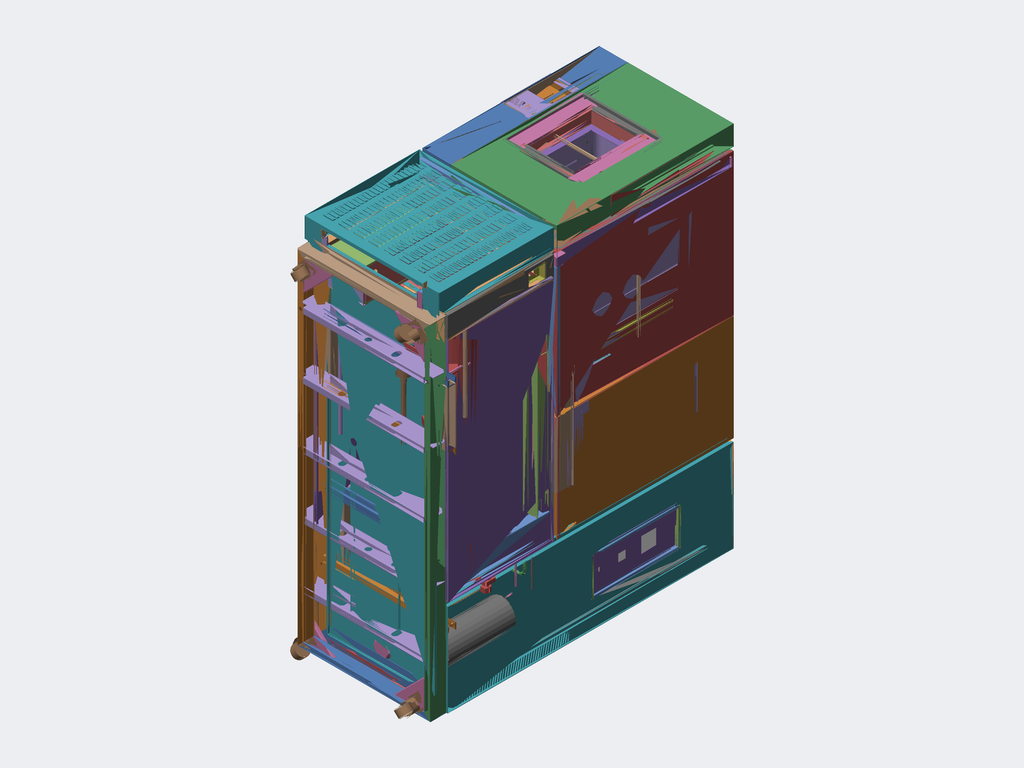Assembly | STEP file | 165 different items | 941 placed
Parts list (item | name | quantity | parent item | size | volume):
1 | HESS-408-70-15W-W-1-outer case side panel 1 | x1 | in HESS-408-70-15W-outer case assembly | 798.5 x 1049 x 630 mm | 1988997 mm3
2 | HESS-408-70-15W-W-2-outer case side panel 2 | x1 | in HESS-408-70-15W-outer case assembly | 798.5 x 1049 x 630 mm | 1938320 mm3
3 | HESS-408-70-15W-W-3-outer case side panel 3 | x1 | in HESS-408-70-15W-outer case assembly | 798.5 x 1049 x 850 mm | 2623190 mm3
4 | HESS-408-70-15W-W-4-outer case side panel 4 | x1 | in HESS-408-70-15W-outer case assembly | 798.5 x 1049 x 850 mm | 2624739 mm3
5 | HESS-408-70-15W-W-5-outer case reinforcing rib 1 | x1 | in HESS-408-70-15W-outer case assembly | 1043 x 80 x 20 mm | 296450 mm3
6 | HESS-408-70-15W-W-6-outer case reinforcing rib 2 | x1 | in HESS-408-70-15W-outer case assembly | 20 x 1043 x 80 mm | 295868 mm3
7 | HESS-408-70-15W-W-7-outer case reinforcing rib 3 | x2 | in HESS-408-70-15W-outer case assembly | 790 x 58.5 x 64 mm | 256348 mm3
8 | HESS-408-70-15W-W-8-outer case reinforcing rib 4 | x2 | in HESS-408-70-15W-outer case assembly | 45 x 930 x 20 mm | 171064 mm3
9 | HESS-408-70-15W-W-9-outer case triangular plate | x4 | in HESS-408-70-15W-outer case assembly | 60 x 60 x 4 mm | 2733 mm3
10 | HESS-408-70-15W-W-10-outer case rear closing plate | x1 | in HESS-408-70-15W-outer case assembly | 697 x 947 x 15 mm | 1092654 mm3
11 | HESS-408-70-15W-W-38-motor fixing bracket | x1 | in HESS-408-70-15W-outer case assembly | 795 x 36 x 250 mm | 812268 mm3
12 | HESS-408-70-15W-W-46-outer case reinforcing rib 5 | x2 | in HESS-408-70-15W-outer case assembly | 755 x 18.5 x 60 mm | 169016 mm3
13 | HESS-408-70-15W-W-47-outer case reinforcing rib 6 | x1 | in HESS-408-70-15W-outer case assembly | 670 x 18.5 x 34 mm | 97679 mm3
14 | HESS-408-70-15W-W-48-outer case reinforcing rib 7 | x2 | in HESS-408-70-15W-outer case assembly | 620 x 18 x 60 mm | 138005 mm3
15 | HESS-408-70-15W-N-1-inner liner upper cover | x1 | in HESS-408-70-15W-inner liner assembly | 650 x 790 x 1338 mm | 2883753 mm3
16 | HESS-408-70-15W-N-2-inner liner lower cover | x1 | in HESS-408-70-15W-inner liner assembly | 650 x 110 x 1338 mm | 1081692 mm3
17 | HESS-408-70-15W-N-3-inner liner rear panel | x1 | in HESS-408-70-15W-inner liner assembly | 600 x 864.78 x 10 mm | 539176 mm3
18 | HESS-408-70-15W-N-6-inner liner turbine outlet baffle | x1 | in HESS-408-70-15W-inner liner assembly | 600 x 69 x 169 mm | 141384 mm3
19 | HESS-408-70-15W-N-7-inner liner turbine panel | x1 | in HESS-408-70-15W-inner liner assembly | 492.743 x 461.634 x 1 mm | 101400 mm3
20 | HESS-408-70-15W-N-8-inner liner turbine enclosure plate | x1 | in HESS-408-70-15W-inner liner assembly | 512.743 x 461.634 x 144 mm | 193062 mm3
21 | HESS-408-70-15W-N-9-inner liner rounded corner | x4 | in HESS-408-70-15W-inner liner assembly | 55 x 55 x 1 mm | 2125 mm3
22 | HESS-408-70-15W-N-12-inner liner closing plate bracket Z | x1 | in HESS-408-70-15W-inner liner assembly | 30 x 657 x 20 mm | 34871 mm3
23 | HESS-408-70-15W-N-11-inner liner closing plate bracket Y | x1 | in HESS-408-70-15W-inner liner assembly | 30 x 657 x 20 mm | 34871 mm3
24 | HESS-408-70-15W-N-13-inner liner outer closing plate | x1 | in HESS-408-70-15W-inner liner assembly | 792 x 1042 x 2.5 mm | 754601 mm3
25 | HESS-408-70-15W-N-14-inner liner partition bracket | x4 | in HESS-408-70-15W-inner liner assembly | 12 x 600 x 42 mm | 43540 mm3
26 | HESS-408-70-15W-N-15-inner liner closing plate | x1 | in HESS-408-70-15W-inner liner assembly | 568 x 685 x 18 mm | 406764 mm3
27 | HESS-408-70-15W-N-16-inner liner louver left side panel | x1 | in HESS-408-70-15W-inner liner louver assembly | 40 x 194 x 15 mm | 10672 mm3
28 | HESS-408-70-15W-N-17-inner liner louver right side panel | x1 | in HESS-408-70-15W-inner liner louver assembly | 40 x 194 x 15 mm | 9821 mm3
29 | HESS-408-70-15W-N-18-inner liner louver blade | x8 | in HESS-408-70-15W-inner liner louver assembly | 516 x 19.734 x 14.16 mm | 12923 mm3
30 | HESS-408-70-15W-N-19-inner liner louver upper baffle | x1 | in HESS-408-70-15W-inner liner louver assembly | 519 x 20 x 2.1 mm | 18114 mm3
31 | HESS-408-70-15W-N-20-inner liner louver lower baffle | x1 | in HESS-408-70-15W-inner liner louver assembly | 519 x 20 x 25 mm | 26517 mm3
32 | HESS-408-70-15W-N-21-inner liner partition plate | x2 | in HESS-408-70-15W-inner liner partition plate assembly | - | 280081 mm3
33 | HESS-408-70-15W-N-22-inner liner partition plate reinforcing rib | x2 | in HESS-408-70-15W-inner liner partition plate assembly | 560 x 13 x 43 mm | 36943 mm3
34 | HESS-408-70-15W-N-23-inner liner bottom plate reinforcing plate 1 | x3 | in HESS-408-70-15W-inner liner assembly | 50 x 540 x 16.5 mm | 59626 mm3
35 | HESS-408-70-15W-D-6-electrical mounting plate bracket | x1 | in HESS-408-70-15W-electrical box assembly | 13 x 43 x 470 mm | 31006 mm3
36 | HESS-408-70-15W-D-4-electrical box bottom plate | x1 | in HESS-408-70-15W-electrical box assembly | 640 x 113.5 x 30 mm | 146678 mm3
37 | HESS-408-70-15W-D-11-frame panel | x1 | in HESS-408-70-15W-electrical box assembly | 1.5 x 520 x 220 mm | 155544 mm3
38 | HESS-408-70-15W-D-2-electrical box right side panel | x1 | in HESS-408-70-15W-electrical box assembly | 93.5 x 1699 x 568.5 mm | 1802522 mm3
39 | HESS-408-70-15W-D-7-electrical box door panel reinforcing rib | x1 | in HESS-408-70-15W-electrical box assembly | 77 x 1495 x 12.5 mm | 218735 mm3
40 | HESS-408-70-15W-D-5-electrical box door panel | x1 | in HESS-408-70-15W-electrical box assembly | 636 x 1516 x 14 mm | 1489085 mm3
41 | HESS-408-70-15W-D-12-electrical mounting plate | x1 | in HESS-408-70-15W-electrical box assembly | 520 x 1630 x 10 mm | 1311169 mm3
42 | HESS-408-70-15W-D-1-electrical box left side panel | x1 | in HESS-408-70-15W-electrical box assembly | 93.5 x 1699 x 568.5 mm | 1630922 mm3
43 | HESS-408-70-15W-D-3-electrical box top plate | x1 | in HESS-408-70-15W-electrical box assembly | 797 x 93.5 x 568.5 mm | 793198 mm3
44 | HESS-408-70-15W-D-10-edge strip 2 | x2 | in HESS-408-70-15W-electrical box frame assembly | 500 x 20 x 15 mm | 30917 mm3
45 | HESS-408-70-15W-D-9-edge strip 1 | x2 | in HESS-408-70-15W-electrical box frame assembly | 230 x 20 x 15 mm | 13161 mm3
46 | HESS-408-70-15W-D-8-electrical box lower closing plate | x1 | in HESS-408-70-15W-electrical box assembly | 200 x 95 x 3 mm | 41690 mm3
47 | HESS-408-70-15W-W-15-bottom frame 5 | x5 | in HESS-408-70-15W-base assembly | 785 x 100 x 50 mm | 395842 mm3
48 | HESS-408-70-15W-W-11-bottom frame 1 | x1 | in HESS-408-70-15W-base assembly | 790 x 100 x 100 mm | 538062 mm3
49 | HESS-408-70-15W-W-12-bottom frame 2 | x1 | in HESS-408-70-15W-base assembly | 790 x 100 x 100 mm | 531868 mm3
50 | HESS-408-70-15W-W-13-bottom frame 3 | x1 | in HESS-408-70-15W-base assembly | 100 x 100 x 2039 mm | 1445665 mm3
51 | HESS-408-70-15W-W-14-bottom frame 4 | x1 | in HESS-408-70-15W-base assembly | 100 x 100 x 2039 mm | 1445666 mm3
52 | HESS-408-70-15W-W-29-outer case lower support 4 | x1 | in HESS-408-70-15W-base assembly | 85 x 100 x 1180 mm | 851335 mm3
53 | HESS-408-70-15W-W-19-side door panel | x2 | in HESS-408-70-15W-base assembly | 18 x 629 x 1358 mm | 1424005 mm3
54 | HESS-408-70-15W-W-20-cabinet lower left outer plate | x1 | in HESS-408-70-15W-base assembly | 21.5 x 631 x 120 mm | 150313 mm3
55 | HESS-408-70-15W-W-18-bottom frame triangular plate | x4 | in HESS-408-70-15W-base assembly | 175 x 18 x 175 mm | 57661 mm3
56 | HESS-408-70-15W-W-21-cabinet lower right outer plate | x1 | in HESS-408-70-15W-base assembly | 21.5 x 631 x 120 mm | 138943 mm3
57 | HESS-408-70-15W-W-30-emergency stop switch box | x1 | in HESS-408-70-15W-base assembly | 35 x 114 x 94 mm | 21062 mm3
58 | HESS-408-70-15W-W-16-bottom frame drip tray 1 | x1 | in HESS-408-70-15W-base assembly | 2000 x 15 x 640 mm | 2094402 mm3
59 | HESS-408-70-15W-W-17-outer case lower support 1 | x1 | in HESS-408-70-15W-base assembly | 763 x 650 x 150 mm | 1372071 mm3
60 | HESS-408-70-15W-W-27-outer case lower support 2 | x1 | in HESS-408-70-15W-base assembly | 763 x 650 x 150 mm | 1289227 mm3
61 | HESS-408-70-15W-W-28-outer case lower support 3 | x1 | in HESS-408-70-15W-base assembly | 85 x 100 x 1180 mm | 851335 mm3
62 | door stop B | x2 | in HESS-408-70-15W-base assembly | 10 x 36.6 x 13.8 mm | 1298 mm3
63 | front lower door bracket-Z (SPCC-3.0) | x1 | in HESS-408-70-15W-base assembly | 30 x 40 x 87 mm | 14354 mm3
64 | copper tube 1_default_machined_ | x1 | in 408 quick-temperature-change freezer tray assembly | 388 x 422 x 519.8 mm | 116086 mm3
65 | VIB-C1-3-8-vibration damping pipe 35_default_machined_ | x2 | in 408 quick-temperature-change freezer tray assembly | 380 x 45 x 45 mm | 185668 mm3
66 | 4NES-14Y-40P | x1 | in 408 quick-temperature-change freezer tray assembly | - | -
67 | copper tube 3_default_machined_ | x1 | in 408 quick-temperature-change freezer tray assembly | 235 x 205.85 x 207.5 mm | 114578 mm3
68 | copper tube 5_default_machined_ | x1 | in 408 quick-temperature-change freezer tray assembly | 35 x 22 x 22 mm | 3381 mm3
69 | SGN22S-sight glass | x1 | in 408 quick-temperature-change freezer tray assembly | 173 x 36.5 x 29 mm | 27166 mm3
70 | three-quarters elbow_default_machined_ | x2 | in 408 quick-temperature-change freezer tray assembly | 35 x 19 x 35 mm | 3675 mm3
71 | copper tube 4_default_machined_ | x1 | in 408 quick-temperature-change freezer tray assembly | 1681 x 220 x 205.42 mm | 263812 mm3
72 | 4PES-12Y-40P | x1 | in 408 quick-temperature-change freezer tray assembly | - | -
73 | TL42B-88D-1-plate heat exchanger 1 | x1 | in TL42B-88D plate heat exchanger assembly | 200 x 460 x 210 mm | 296477 mm3
74 | TL42B-88D-3-plate heat exchanger 3 | x1 | in TL42B-88D plate heat exchanger assembly | 198 x 458 x 1 mm | 84209 mm3
75 | TL42B-88D-2-plate heat exchanger 2 | x2 | in TL42B-88D plate heat exchanger assembly | 198 x 15 x 209 mm | 51964 mm3
76 | HESS-408-70-15W-W-39-5# channel 1_default_machined_ | x4 | in HESS-408-70-15W-base channel assembly 2, HESS-408-70-15W-base channel assembly 1 | 330 x 50 x 37 mm | 223683 mm3
77 | HESS-408-70-15W-W-41-5# channel 3_default_machined_ | x2 | in HESS-408-70-15W-base channel assembly 2, HESS-408-70-15W-base channel assembly 1 | 37 x 50 x 740 mm | 491245 mm3
78 | HESS-408-70-15W-W-40-5# channel 2_default_machined_ | x2 | in HESS-408-70-15W-base channel assembly 2, HESS-408-70-15W-base channel assembly 1 | 37 x 50 x 740 mm | 497631 mm3
79 | 10+13RT condenser | x1 | in 408 quick-temperature-change freezer tray assembly | 263 x 339 x 1390 mm | 54968408 mm3
80 | copper tube 2_default_machined_ | x1 | in 408 quick-temperature-change freezer tray assembly | 129.5 x 170 x 302.5 mm | 90840 mm3
81 | PN_0001-1-1-8-oil separator 28 | x1 | in 408 quick-temperature-change freezer tray assembly | 100 x 435 x 100 mm | 2983083 mm3
82 | TPLC-844-eight-litre receiver tank | x1 | in 408 quick-temperature-change freezer tray assembly | 170 x 466.103 x 170 mm | 9402386 mm3
83 | 4PES-12Y-40P-1 | x1 | in 408 quick-temperature-change freezer tray assembly | 176.41 x 90.99 x 84 mm | 162399 mm3
84 | one-inch elbow_default_machined_ | x2 | in 408 quick-temperature-change freezer tray assembly | 40.4 x 25 x 40.4 mm | 3722 mm3
85 | copper tube 8_default_machined_ | x1 | in 408 quick-temperature-change freezer tray assembly | 80 x 22 x 22 mm | 7728 mm3
86 | copper tube 9_default_machined_ | x1 | in 408 quick-temperature-change freezer tray assembly | 35 x 16 x 16 mm | 2392 mm3
87 | copper tube 12_default_machined_ | x1 | in 408 quick-temperature-change freezer tray assembly | 109.5 x 122.5 x 899.3 mm | 84690 mm3
88 | copper tube 13_default_machined_ | x1 | in 408 quick-temperature-change freezer tray assembly | 110 x 22 x 22 mm | 10626 mm3
89 | VIB-C1-1-8-vibration damping pipe 28_default_machined_ | x2 | in 408 quick-temperature-change freezer tray assembly | 340 x 35 x 35 mm | 105306 mm3
90 | copper tube 10_default_machined_ | x1 | in 408 quick-temperature-change freezer tray assembly | 157.296 x 118.586 x 16 mm | 14200 mm3
91 | copper tube 17_default_machined_ | x1 | in 408 quick-temperature-change freezer tray assembly | 314 x 114 x 28 mm | 47271 mm3
92 | copper tube 6_default_machined_ | x1 | in 408 quick-temperature-change freezer tray assembly | 91 x 141 x 22 mm | 18214 mm3
93 | EK-167S-seven-eighths filter | x2 | in 408 quick-temperature-change freezer tray assembly | 180 x 67 x 67 mm | 48133 mm3
94 | copper tube 7_default_machined_ | x1 | in 408 quick-temperature-change freezer tray assembly | 217.778 x 178.778 x 22 mm | 26481 mm3
95 | five-eighths elbow_default_machined_ | x1 | in 408 quick-temperature-change freezer tray assembly | 30 x 16 x 30 mm | 1831 mm3
96 | DX3-012-electronic expansion valve | x1 | in 408 quick-temperature-change freezer tray assembly | 26 x 143.6 x 91 mm | 49456 mm3
97 | copper tube 11_default_machined_ | x1 | in 408 quick-temperature-change freezer tray assembly | 248 x 88 x 16 mm | 20399 mm3
98 | seven-eighths solenoid valve | x1 | in 408 quick-temperature-change freezer tray assembly | 189.5 x 104.6 x 71.674 mm | 229538 mm3
99 | copper tube 14_default_machined_ | x1 | in 408 quick-temperature-change freezer tray assembly | 294.5 x 148 x 164 mm | 63386 mm3
100 | copper tube 15_default_machined_ | x1 | in 408 quick-temperature-change freezer tray assembly | 627.9 x 174 x 28 mm | 93963 mm3
101 | copper tube 16_default_machined_ | x1 | in 408 quick-temperature-change freezer tray assembly | 191.58 x 28 x 183.16 mm | 49168 mm3
102 | copper tube 21_default_machined_ | x1 | in 408 quick-temperature-change freezer tray assembly | 351.2 x 586 x 22 mm | 82193 mm3
103 | SEV-1506DYF-three-quarter inlet solenoid valve | x2 | in 408 quick-temperature-change freezer tray assembly | 190 x 114 x 54 mm | 186702 mm3
104 | copper tube 29_default_machined_ | x1 | in copper tube group 01 | 153.175 x 53.175 x 6.35 mm | 2610 mm3
105 | quarter tee_default_machined_ | x2 | in copper tube group 01 | 25.4 x 16 x 8 mm | 593.284 mm3
106 | copper tube 33_default_machined_ | x1 | in copper tube group 01 | 328.675 x 183.099 x 47.35 mm | 11843 mm3
107 | copper tube 30_default_machined_ | x1 | in copper tube group 01 | 66.35 x 153.175 x 256.35 mm | 6515 mm3
108 | 1-4 solenoid valve | x1 | in copper tube group 01 | 14 x 71 x 42 mm | 5783 mm3
109 | copper tube 27_default_machined_ | x1 | in copper tube group 01 | 6.35 x 100 x 6.35 mm | 1395 mm3
110 | copper tube 31_default_machined_ | x1 | in copper tube group 01 | 172 x 6.35 x 6.35 mm | 2399 mm3
111 | copper tube 26_default_machined_ | x1 | in copper tube group 01 | 123.175 x 103.175 x 6.35 mm | 2919 mm3
112 | SEV-603DXF-3-8-cooling solenoid valve | x2 | in copper tube group 01, 408 quick-temperature-change freezer tray assembly | 138 x 39 x 64 mm | 65143 mm3
113 | copper tube 28_default_machined_ | x1 | in copper tube group 01 | 50 x 6.35 x 6.35 mm | 697.434 mm3
114 | copper tube 32_default_machined_ | x1 | in copper tube group 01 | 40 x 6.35 x 6.35 mm | 557.947 mm3
115 | 2.5 capillary tube | x3 | in copper tube group 01, 408 quick-temperature-change freezer tray assembly | 85.019 x 52 x 19.082 mm | 4215 mm3
116 | cooling electronic expansion valve | x1 | in copper tube group 01 | 54.65 x 97.5 x 17.3 mm | 14688 mm3
117 | liquid charging valve head | x1 | in 408 quick-temperature-change freezer tray assembly | 12.471 x 10.8 x 44.796 mm | 1804 mm3
118 | copper tube 22_default_machined_ | x1 | in 408 quick-temperature-change freezer tray assembly | 787.8 x 486 x 195 mm | 412220 mm3
119 | copper tube 20_default_machined_ | x1 | in 408 quick-temperature-change freezer tray assembly | 340 x 22 x 22 mm | 32845 mm3
120 | copper tube 18_default_machined_ | x1 | in 408 quick-temperature-change freezer tray assembly | 1334 x 414.525 x 49.525 mm | 41948 mm3
121 | copper tube 25_default_machined_ | x1 | in 408 quick-temperature-change freezer tray assembly | 374.675 x 273.558 x 413.267 mm | 42436 mm3
122 | copper tube 19_default_machined_ | x1 | in 408 quick-temperature-change freezer tray assembly | 638.85 x 402.7 x 54.675 mm | 25549 mm3
123 | copper tube 23_default_machined_ | x1 | in 408 quick-temperature-change freezer tray assembly | 108 x 489 x 88 mm | 42273 mm3
124 | BML18S | x1 | in 408 quick-temperature-change freezer tray assembly | 83 x 90.853 x 130 mm | 164797 mm3
125 | tee copper tube | x1 | in 408 quick-temperature-change freezer tray assembly | 50 x 34.25 x 18.5 mm | 4026 mm3
126 | part 153^evaporator 408 by COMPANY_A | x1 | in 408 evaporator by COMPANY_A | 512 x 433 x 30.095 mm | 277126 mm3
127 | mirrored part 153^COMPANY_A 408 evaporator | x1 | in 408 evaporator by COMPANY_A | 512 x 433 x 30.095 mm | 277126 mm3
128 | part 155^evaporator 408 by COMPANY_A | x320 | in 408 evaporator by COMPANY_A | 10 x 10 x 460 mm | 13006 mm3
129 | part 156^COMPANY_A 408 evaporator | x89 | in 408 evaporator by COMPANY_A | 510.4 x 397 x 0.2 mm | 34444 mm3
130 | connecting copper tube | x160 | in 408 evaporator by COMPANY_A | 35 x 10 x 22.5 mm | 3870 mm3
131 | connecting copper tube 3 | x150 | in 408 evaporator by COMPANY_A | 10 x 23.975 x 37.95 mm | 4234 mm3
132 | part 159^COMPANY_A 408 evaporator | x1 | in 408 evaporator by COMPANY_A | 24.816 x 24.816 x 185 mm | 40377 mm3
133 | part 161^COMPANY_A 408 evaporator | x1 | in 408 evaporator by COMPANY_A | 66.5 x 28 x 545 mm | 366001 mm3
134 | filter | x1 | in 408 quick-temperature-change freezer tray assembly | 40 x 40 x 80 mm | 10214 mm3
135 | copper tube 36 | x1 | in 408 quick-temperature-change freezer tray assembly | 22 x 22 x 50 mm | 19007 mm3
136 | expansion valve | x1 | in 408 quick-temperature-change freezer tray assembly | 79 x 143.2 x 26 mm | 54651 mm3
137 | copper tube 37 | x1 | in 408 quick-temperature-change freezer tray assembly | 261.823 x 291.69 x 49.416 mm | 86044 mm3
138 | stop valve | x1 | in 408 quick-temperature-change freezer tray assembly | 130 x 21.6 x 21.6 mm | 7854 mm3
139 | capillary tube extension | x1 | in 408 quick-temperature-change freezer tray assembly | 2 x 2 x 30 mm | 94.248 mm3
140 | right-angle cylinder elbow | x2 | in 408 quick-temperature-change freezer tray assembly | 81.8 x 81.8 x 37.6 mm | 14457 mm3
141 | copper tube 41 | x1 | in 408 quick-temperature-change freezer tray assembly | 35 x 35 x 250 mm | 31856 mm3
142 | copper tube 42_default_machined_ | x1 | in 408 quick-temperature-change freezer tray assembly | 63.3 x 483.405 x 112.3 mm | 215626 mm3
143 | copper tube 44 | x1 | in 408 quick-temperature-change freezer tray assembly | 53 x 16 x 106 mm | 7500 mm3
144 | copper tube 45_default_machined_ | x1 | in 408 quick-temperature-change freezer tray assembly | 16 x 79.107 x 16 mm | 15905 mm3
145 | copper tube 46_default_machined_ | x1 | in 408 quick-temperature-change freezer tray assembly | 241 x 728.501 x 256 mm | 124522 mm3
146 | joint | x3 | in 408 quick-temperature-change freezer tray assembly | 8.5 x 10 x 8.5 mm | 235.619 mm3
147 | SK6-U75105BP-3 inch heavy-duty caster | x4 | in HESS-408-70-15W-base assembly | 114.176 x 105 x 81 mm | 325491 mm3
148 | Front lower door bracket-Y (SPCC-3.0) | x1 | in HESS-408-70-15W-base assembly | 30 x 40 x 87 mm | 14350 mm3
149 | damper support B | x1 | in HESS-408-70-15W-base assembly | 24 x 46 x 18 mm | 2428 mm3
150 | HESS-408-70-15W-W-25-lower door support bracket 2 | x1 | in HESS-408-70-15W-lower door assembly | 21.5 x 75.5 x 23.5 mm | 6756 mm3
151 | HESS-408-70-15W-W-22-lower door frame | x1 | in HESS-408-70-15W-lower door assembly | 800 x 681 x 144 mm | 1412616 mm3
152 | HESS-408-70-15W-W-23-lower door frame support plate | x2 | in HESS-408-70-15W-lower door assembly | 3 x 25 x 137 mm | 9662 mm3
153 | HESS-408-70-15W-W-26-lower door drip tray | x1 | in HESS-408-70-15W-lower door assembly | 776 x 23 x 106 mm | 113085 mm3
154 | HESS-408-70-15W-W-24-lower door support bracket | x1 | in HESS-408-70-15W-lower door assembly | 21.5 x 130 x 23.5 mm | 11618 mm3
155 | HESS-408-70-15W-W-37-upper door glass inner frame 3 | x2 | in HESS-408-70-15W-glass inner frame assembly 1 | 365 x 466.5 x 97 mm | 170617 mm3
156 | HESS-408-70-15W-W-34-front control panel | x1 | in HESS-408-70-15W-upper door assembly | 170 x 310 x 1.5 mm | 47327 mm3
157 | HESS-408-70-15W-W-44-upper door left reinforcing plate | x1 | in HESS-408-70-15W-upper door assembly | 3 x 980 x 110 mm | 321603 mm3
158 | HESS-408-70-15W-W-31-upper door left frame | x1 | in HESS-408-70-15W-upper door assembly | 170 x 1050 x 120 mm | 637779 mm3
159 | HESS-408-70-15W-W-33-front door electrical control box | x1 | in HESS-408-70-15W-upper door assembly | 158 x 50 x 302 mm | 132853 mm3
160 | HESS-408-70-15W-W-32-upper door right frame | x1 | in HESS-408-70-15W-upper door assembly | 630 x 1050 x 120 mm | 1382847 mm3
161 | HESS-408-70-15W-W-45-upper door right reinforcing plate | x1 | in HESS-408-70-15W-upper door assembly | 3 x 400 x 110 mm | 131875 mm3
162 | HESS-408-70-15W-W-43-upper door closing plate 2 | x1 | in HESS-408-70-15W-upper door assembly | 380 x 480 x 2.5 mm | 187480 mm3
163 | HESS-408-70-15W-W-42-upper door closing plate 1 | x1 | in HESS-408-70-15W-upper door assembly | 796 x 1046 x 1.5 mm | 1022602 mm3
164 | HESS-408-70-15W-W-35-upper door glass inner frame 1 | x2 | in HESS-408-70-15W-upper door glass inner frame assembly 2 | 465 x 101 x 20 mm | 97847 mm3
165 | HESS-408-70-15W-W-36-upper door glass inner frame 2 | x2 | in HESS-408-70-15W-upper door glass inner frame assembly 2 | 51 x 462 x 20 mm | 47605 mm3
Placements (level | parent | child | x y z in mm | rotation matrix by rows), first 228 of 960 lines:
1 | HESS-408-70-15W-quick-temperature-change cabinet assembly | HESS-408-70-15W-outer case assembly | -21.786 122.921 6.0 | 1 0 0 0 1 0 0 0 1
2 | HESS-408-70-15W-outer case assembly | HESS-408-70-15W-W-1-outer case side panel 1 | -195.793 637.671 1049.0 | 1 0 0 0 1 0 0 0 1
2 | HESS-408-70-15W-outer case assembly | HESS-408-70-15W-W-2-outer case side panel 2 | -194.293 -410.829 1049.0 | 1 0 0 0 1 0 0 0 1
2 | HESS-408-70-15W-outer case assembly | HESS-408-70-15W-W-3-outer case side panel 3 | -195.793 637.671 1789.0 | 1 0 0 0 1 0 0 0 1
2 | HESS-408-70-15W-outer case assembly | HESS-408-70-15W-W-4-outer case side panel 4 | -194.293 -410.829 1789.0 | 1 0 0 0 1 0 0 0 1
2 | HESS-408-70-15W-outer case assembly | HESS-408-70-15W-W-5-outer case reinforcing rib 1 | 200.457 112.671 2172.0 | 0 0 -1 -1 0 0 0 1 0
2 | HESS-408-70-15W-outer case assembly | HESS-408-70-15W-W-6-outer case reinforcing rib 2 | -590.543 112.671 2172.0 | 1 0 0 0 1 0 0 0 1
2 | HESS-408-70-15W-outer case assembly | HESS-408-70-15W-W-7-outer case reinforcing rib 3 | -590.043 -352.329 2199.0 | 1 0 0 0 1 0 0 0 1
2 | HESS-408-70-15W-outer case assembly | HESS-408-70-15W-W-7-outer case reinforcing rib 3 | 199.957 577.671 2199.0 | -1 0 0 0 -1 0 0 0 1
2 | HESS-408-70-15W-outer case assembly | HESS-408-70-15W-W-8-outer case reinforcing rib 4 | 144.957 112.671 2199.0 | 1 0 0 0 1 0 0 0 1
2 | HESS-408-70-15W-outer case assembly | HESS-408-70-15W-W-8-outer case reinforcing rib 4 | -535.043 112.671 2199.0 | -1 0 0 0 -1 0 0 0 1
2 | HESS-408-70-15W-outer case assembly | HESS-408-70-15W-W-9-outer case triangular plate | 154.957 587.671 749.0 | -1 0 0 0 1 0 0 0 -1
2 | HESS-408-70-15W-outer case assembly | HESS-408-70-15W-W-9-outer case triangular plate | -545.043 587.671 749.0 | 0 -1 0 -1 0 0 0 0 -1
2 | HESS-408-70-15W-outer case assembly | HESS-408-70-15W-W-9-outer case triangular plate | -545.043 -362.329 749.0 | 1 0 0 0 -1 0 0 0 -1
2 | HESS-408-70-15W-outer case assembly | HESS-408-70-15W-W-9-outer case triangular plate | 154.957 -362.329 749.0 | 0 1 0 1 0 0 0 0 -1
2 | HESS-408-70-15W-outer case assembly | HESS-408-70-15W-W-10-outer case rear closing plate | -195.043 112.671 735.5 | 1 0 0 0 1 0 0 0 1
2 | HESS-408-70-15W-outer case assembly | HESS-408-70-15W-W-38-motor fixing bracket | -165.043 636.171 1144.0 | -1 0 0 0 1 0 0 0 -1
2 | HESS-408-70-15W-outer case assembly | HESS-408-70-15W-W-46-outer case reinforcing rib 5 | -562.043 -407.829 1754.5 | 0 0 1 0 1 0 -1 0 -0
2 | HESS-408-70-15W-outer case assembly | HESS-408-70-15W-W-46-outer case reinforcing rib 5 | 173.457 -407.829 1754.5 | 0 0 -1 0 1 0 1 0 0
2 | HESS-408-70-15W-outer case assembly | HESS-408-70-15W-W-47-outer case reinforcing rib 6 | -195.043 -407.829 752.5 | 1 0 0 0 1 0 0 0 1
2 | HESS-408-70-15W-outer case assembly | HESS-408-70-15W-W-48-outer case reinforcing rib 7 | 173.457 -407.829 1049.0 | 0 0 -1 0 1 0 1 0 0
2 | HESS-408-70-15W-outer case assembly | HESS-408-70-15W-W-48-outer case reinforcing rib 7 | -562.043 -407.829 1049.0 | 0 0 1 0 1 0 -1 0 -0
1 | HESS-408-70-15W-quick-temperature-change cabinet assembly | HESS-408-70-15W-inner liner assembly | -170.815 170.854 568.0 | 1 0 0 0 1 0 0 0 1
2 | HESS-408-70-15W-inner liner assembly | HESS-408-70-15W-N-1-inner liner upper cover | -46.013 -275.261 983.0 | 1 0 0 0 1 0 0 0 1
2 | HESS-408-70-15W-inner liner assembly | HESS-408-70-15W-N-2-inner liner lower cover | -46.013 -275.261 983.0 | 1 0 0 0 1 0 0 0 1
2 | HESS-408-70-15W-inner liner assembly | HESS-408-70-15W-N-3-inner liner rear panel | -46.013 -275.261 314.0 | 1 0 0 0 1 0 0 0 1
2 | HESS-408-70-15W-inner liner assembly | HESS-408-70-15W-N-6-inner liner turbine outlet baffle | -46.013 414.739 798.0 | 1 0 0 0 0 -1 0 1 0
2 | HESS-408-70-15W-inner liner assembly | HESS-408-70-15W-N-7-inner liner turbine panel | -2094.29 344.739 -316.641 | 1 0 0 0 0 -1 0 1 0
2 | HESS-408-70-15W-inner liner assembly | HESS-408-70-15W-N-8-inner liner turbine enclosure plate | -2094.29 417.739 -316.641 | 1 0 0 0 0 -1 0 1 0
2 | HESS-408-70-15W-inner liner assembly | HESS-408-70-15W-N-9-inner liner rounded corner | 223.987 459.739 1652.0 | 1 0 0 0 1 0 0 0 1
2 | HESS-408-70-15W-inner liner assembly | HESS-408-70-15W-N-9-inner liner rounded corner | -316.013 459.739 1652.0 | 0 -1 0 1 0 0 0 0 1
2 | HESS-408-70-15W-inner liner assembly | HESS-408-70-15W-N-9-inner liner rounded corner | -316.013 -330.259 1652.0 | -1 0 0 0 -1 0 0 0 1
2 | HESS-408-70-15W-inner liner assembly | HESS-408-70-15W-N-9-inner liner rounded corner | 223.987 -330.259 1652.0 | 0 1 0 -1 0 0 0 0 1
2 | HESS-408-70-15W-inner liner assembly | HESS-408-70-15W-N-12-inner liner closing plate bracket Z | -338.513 -8.761 852.0 | 1 0 0 0 1 0 0 0 1
2 | HESS-408-70-15W-inner liner assembly | HESS-408-70-15W-N-11-inner liner closing plate bracket Y | 246.487 -8.761 852.0 | 1 0 0 0 1 0 0 0 1
2 | HESS-408-70-15W-inner liner assembly | HESS-408-70-15W-N-13-inner liner outer closing plate | -46.013 64.739 1657.0 | 1 0 0 0 1 0 0 0 1
2 | HESS-408-70-15W-inner liner assembly | HESS-408-70-15W-N-14-inner liner partition bracket | -334.013 29.739 1561.0 | 1 0 0 0 1 0 0 0 1
2 | HESS-408-70-15W-inner liner assembly | HESS-408-70-15W-N-14-inner liner partition bracket | -334.013 29.739 943.0 | 1 0 0 0 1 0 0 0 1
2 | HESS-408-70-15W-inner liner assembly | HESS-408-70-15W-N-14-inner liner partition bracket | 241.987 29.739 1561.0 | -1 0 0 0 1 0 0 0 -1
2 | HESS-408-70-15W-inner liner assembly | HESS-408-70-15W-N-14-inner liner partition bracket | 241.987 29.739 943.0 | -1 0 0 0 1 0 0 0 -1
2 | HESS-408-70-15W-inner liner assembly | HESS-408-70-15W-N-15-inner liner closing plate | -46.013 -22.761 849.1 | 1 0 0 0 1 0 0 0 1
2 | HESS-408-70-15W-inner liner assembly | HESS-408-70-15W-inner liner louver assembly | -283.743 462.245 759.459 | 1 0 0 0 0.866 -0.5 0 0.5 0.866
3 | HESS-408-70-15W-inner liner louver assembly | HESS-408-70-15W-N-16-inner liner louver left side panel | -41.77 21.581 151.5 | 1 0 0 0 1 0 0 0 1
3 | HESS-408-70-15W-inner liner louver assembly | HESS-408-70-15W-N-17-inner liner louver right side panel | 517.23 21.581 150.5 | -1 0 0 0 1 0 0 0 -1
3 | HESS-408-70-15W-inner liner louver assembly | HESS-408-70-15W-N-18-inner liner louver blade | 236.73 -70.154 141.045 | 1 0 0 0 0.6428 0.766 0 -0.766 0.6428
3 | HESS-408-70-15W-inner liner louver assembly | HESS-408-70-15W-N-19-inner liner louver upper baffle | 237.73 112.013 143.224 | 1 0 0 0 0.5 -0.866 0 0.866 0.5
3 | HESS-408-70-15W-inner liner louver assembly | HESS-408-70-15W-N-20-inner liner louver lower baffle | 237.73 -65.129 146.884 | -1 0 0 0 -0.866 0.5 0 0.5 0.866
3 | HESS-408-70-15W-inner liner louver assembly | HESS-408-70-15W-N-18-inner liner louver blade | 236.73 -49.154 141.045 | 1 0 0 0 0.6428 0.766 0 -0.766 0.6428
3 | HESS-408-70-15W-inner liner louver assembly | HESS-408-70-15W-N-18-inner liner louver blade | 236.73 -28.154 141.045 | 1 0 0 0 0.6428 0.766 0 -0.766 0.6428
3 | HESS-408-70-15W-inner liner louver assembly | HESS-408-70-15W-N-18-inner liner louver blade | 236.73 -7.154 141.045 | 1 0 0 0 0.6428 0.766 0 -0.766 0.6428
3 | HESS-408-70-15W-inner liner louver assembly | HESS-408-70-15W-N-18-inner liner louver blade | 236.73 13.846 141.045 | 1 0 0 0 0.6428 0.766 0 -0.766 0.6428
3 | HESS-408-70-15W-inner liner louver assembly | HESS-408-70-15W-N-18-inner liner louver blade | 236.73 34.846 141.045 | 1 0 0 0 0.6428 0.766 0 -0.766 0.6428
3 | HESS-408-70-15W-inner liner louver assembly | HESS-408-70-15W-N-18-inner liner louver blade | 236.73 55.846 141.045 | 1 0 0 0 0.6428 0.766 0 -0.766 0.6428
3 | HESS-408-70-15W-inner liner louver assembly | HESS-408-70-15W-N-18-inner liner louver blade | 236.73 76.846 141.045 | 1 0 0 0 0.6428 0.766 0 -0.766 0.6428
2 | HESS-408-70-15W-inner liner assembly | HESS-408-70-15W-inner liner partition plate assembly | -6.366 -309.94 461.999 | 1 0 0 0 1 0 0 0 1
3 | HESS-408-70-15W-inner liner partition plate assembly | HESS-408-70-15W-N-21-inner liner partition plate | -39.647 70.179 790.001 | 1 0 0 0 1 0 0 0 1
3 | HESS-408-70-15W-inner liner partition plate assembly | HESS-408-70-15W-N-22-inner liner partition plate reinforcing rib | -39.647 56.179 790.001 | 1 0 0 0 1 0 0 0 1
2 | HESS-408-70-15W-inner liner assembly | HESS-408-70-15W-inner liner partition plate assembly | -6.366 82.06 461.999 | 1 0 0 0 1 0 0 0 1
3 | HESS-408-70-15W-inner liner partition plate assembly | HESS-408-70-15W-N-21-inner liner partition plate | -39.647 70.179 790.001 | 1 0 0 0 1 0 0 0 1
3 | HESS-408-70-15W-inner liner partition plate assembly | HESS-408-70-15W-N-22-inner liner partition plate reinforcing rib | -39.647 56.179 790.001 | 1 0 0 0 1 0 0 0 1
2 | HESS-408-70-15W-inner liner assembly | HESS-408-70-15W-N-23-inner liner bottom plate reinforcing plate 1 | -46.013 -391.583 419.19 | 0 -1 0 -0.01121 0 0.9999 -0.9999 0 -0.01121
2 | HESS-408-70-15W-inner liner assembly | HESS-408-70-15W-N-23-inner liner bottom plate reinforcing plate 1 | -46.013 -385.081 999.153 | 0 -1 0 -0.01121 0 0.9999 -0.9999 0 -0.01121
2 | HESS-408-70-15W-inner liner assembly | HESS-408-70-15W-N-23-inner liner bottom plate reinforcing plate 1 | -46.013 -378.579 1579.117 | 0 -1 0 -0.01121 0 0.9999 -0.9999 0 -0.01121
1 | HESS-408-70-15W-quick-temperature-change cabinet assembly | HESS-408-70-15W-electrical box assembly | -167.109 -185.713 2154.25 | -1 0 0 0 1 0 0 0 -1
2 | HESS-408-70-15W-electrical box assembly | HESS-408-70-15W-D-6-electrical mounting plate bracket | 435.22 668.806 1679.25 | -1 0 0 0 1 0 0 0 -1
2 | HESS-408-70-15W-electrical box assembly | HESS-408-70-15W-D-4-electrical box bottom plate | 49.72 -703.694 1982.75 | 1 0 0 0 1 0 0 0 1
2 | HESS-408-70-15W-electrical box assembly | HESS-408-70-15W-D-11-frame panel | -330.28 364.806 1707.75 | 1 0 0 0 1 0 0 0 1
2 | HESS-408-70-15W-electrical box assembly | HESS-408-70-15W-D-2-electrical box right side panel | 449.72 95.556 1707.75 | 1 0 0 0 1 0 0 0 1
2 | HESS-408-70-15W-electrical box assembly | HESS-408-70-15W-D-7-electrical box door panel reinforcing rib | 50.22 106.306 1968.75 | 1 0 0 0 1 0 0 0 1
2 | HESS-408-70-15W-electrical box assembly | HESS-408-70-15W-D-5-electrical box door panel | 50.22 106.306 1981.25 | -1 0 0 0 1 0 0 0 -1
2 | HESS-408-70-15W-electrical box assembly | HESS-408-70-15W-D-12-electrical mounting plate | 433.72 118.306 1695.25 | 0 0 -1 0 1 0 1 0 -0
2 | HESS-408-70-15W-electrical box assembly | HESS-408-70-15W-D-1-electrical box left side panel | -348.78 95.556 1707.75 | 1 0 0 0 1 0 0 0 1
2 | HESS-408-70-15W-electrical box assembly | HESS-408-70-15W-D-3-electrical box top plate | 49.72 946.306 1707.75 | 1 0 0 0 1 0 0 0 1
2 | HESS-408-70-15W-electrical box assembly | HESS-408-70-15W-electrical box frame assembly | -318.372 852.306 1735.746 | 0 -1 0 0 0 -1 1 0 0
3 | HESS-408-70-15W-electrical box frame assembly | HESS-408-70-15W-D-10-edge strip 2 | -135.496 33.409 487.5 | 0 0 1 0 1 0 -1 0 -0
3 | HESS-408-70-15W-electrical box frame assembly | HESS-408-70-15W-D-10-edge strip 2 | 79.504 33.409 487.5 | 0 0 -1 0 1 0 1 0 0
3 | HESS-408-70-15W-electrical box frame assembly | HESS-408-70-15W-D-9-edge strip 1 | -27.997 33.409 745.0 | -1 0 0 0 1 0 0 0 -1
3 | HESS-408-70-15W-electrical box frame assembly | HESS-408-70-15W-D-9-edge strip 1 | -27.997 33.409 230.0 | 1 0 0 0 1 0 0 0 1
2 | HESS-408-70-15W-electrical box assembly | HESS-408-70-15W-D-8-electrical box lower closing plate | -98.53 -703.694 1985.75 | 1 0 0 0 1 0 0 0 1
1 | HESS-408-70-15W-quick-temperature-change cabinet assembly | HESS-408-70-15W-base assembly | 115.778 -1086.862 1380.0 | 1 0 0 0 1 0 0 0 1
2 | HESS-408-70-15W-base assembly | HESS-408-70-15W-W-15-bottom frame 5 | -332.607 95.455 -883.5 | 1 0 0 0 1 0 0 0 1
2 | HESS-408-70-15W-base assembly | HESS-408-70-15W-W-11-bottom frame 1 | -332.607 147.455 740.0 | 1 0 0 0 1 0 0 0 1
2 | HESS-408-70-15W-base assembly | HESS-408-70-15W-W-12-bottom frame 2 | -332.607 147.455 -1105.0 | -1 0 0 0 1 0 0 0 -1
2 | HESS-408-70-15W-base assembly | HESS-408-70-15W-W-13-bottom frame 3 | -627.607 147.455 -182.5 | 1 0 0 0 1 0 0 0 1
2 | HESS-408-70-15W-base assembly | HESS-408-70-15W-W-14-bottom frame 4 | -37.607 147.455 -182.5 | -1 0 0 0 1 0 0 0 -1
2 | HESS-408-70-15W-base assembly | HESS-408-70-15W-W-29-outer case lower support 4 | -714.107 747.455 100.0 | -1 0 0 0 1 0 0 0 -1
2 | HESS-408-70-15W-base assembly | HESS-408-70-15W-W-19-side door panel | -732.607 463.955 39.0 | -1 0 0 0 1 0 0 0 -1
2 | HESS-408-70-15W-base assembly | HESS-408-70-15W-W-20-cabinet lower left outer plate | -731.107 462.955 780.0 | 1 0 0 0 1 0 0 0 1
2 | HESS-408-70-15W-base assembly | HESS-408-70-15W-W-18-bottom frame triangular plate | -691.607 47.455 804.0 | 0 0 1 0 -1 0 1 0 0
2 | HESS-408-70-15W-base assembly | HESS-408-70-15W-W-18-bottom frame triangular plate | -691.607 47.455 -1169.0 | -1 0 0 0 -1 0 0 0 1
2 | HESS-408-70-15W-base assembly | HESS-408-70-15W-W-21-cabinet lower right outer plate | 67.393 462.955 780.0 | 1 0 0 0 1 0 0 0 1
2 | HESS-408-70-15W-base assembly | HESS-408-70-15W-W-18-bottom frame triangular plate | 26.393 47.455 804.0 | 1 0 0 0 -1 0 0 0 -1
2 | HESS-408-70-15W-base assembly | HESS-408-70-15W-W-30-emergency stop switch box | 31.893 678.455 780.0 | 1 0 0 0 1 0 0 0 1
2 | HESS-408-70-15W-base assembly | HESS-408-70-15W-W-18-bottom frame triangular plate | 26.393 47.455 -1169.0 | 0 0 -1 0 -1 0 -1 0 -0
2 | HESS-408-70-15W-base assembly | HESS-408-70-15W-W-16-bottom frame drip tray 1 | -332.607 148.955 -160.0 | 0 0 1 0 1 0 -1 0 -0
2 | HESS-408-70-15W-base assembly | HESS-408-70-15W-W-17-outer case lower support 1 | -332.607 797.455 765.0 | -1 0 0 0 1 0 0 0 -1
2 | HESS-408-70-15W-base assembly | HESS-408-70-15W-W-27-outer case lower support 2 | -332.607 797.455 -565.0 | -1 0 0 0 1 0 0 0 -1
2 | HESS-408-70-15W-base assembly | HESS-408-70-15W-W-28-outer case lower support 3 | 48.893 747.455 100.0 | 1 0 0 0 1 0 0 0 1
2 | HESS-408-70-15W-base assembly | HESS-408-70-15W-W-19-side door panel | 67.393 463.955 39.0 | 1 0 0 0 1 0 0 0 1
2 | HESS-408-70-15W-base assembly | door stop B | -685.107 715.705 846.9 | 1 0 0 0 1 0 0 0 1
2 | HESS-408-70-15W-base assembly | front lower door bracket-Z (SPCC-3.0) | -630.607 117.455 884.55 | -1 0 0 0 1 0 0 0 -1
2 | HESS-408-70-15W-base assembly | HESS-408-70-15W-W-15-bottom frame 5 | -332.607 95.455 -164.5 | 1 0 0 0 1 0 0 0 1
2 | HESS-408-70-15W-base assembly | HESS-408-70-15W-W-15-bottom frame 5 | -332.607 95.455 554.5 | 1 0 0 0 1 0 0 0 1
2 | HESS-408-70-15W-base assembly | 408 quick-temperature-change freezer tray assembly | -0.0 -0.0 -0.0 | 1 0 0 0 1 0 0 0 1
3 | 408 quick-temperature-change freezer tray assembly | copper tube 1_default_machined_ | -381.107 568.955 699.8 | 1 0 0 0 1 0 0 0 1
3 | 408 quick-temperature-change freezer tray assembly | VIB-C1-3-8-vibration damping pipe 35_default_machined_ | -294.607 678.955 498.2 | 0 0 1 0 1 0 -1 0 0
3 | 408 quick-temperature-change freezer tray assembly | 4NES-14Y-40P | -494.607 407.601 -610.2 | 0 -1 0 0 0 1 -1 0 0
3 | 408 quick-temperature-change freezer tray assembly | copper tube 3_default_machined_ | -494.608 490.601 -51.8 | 1 0 0 0 1 0 0 0 1
3 | 408 quick-temperature-change freezer tray assembly | copper tube 5_default_machined_ | 5.293 307.936 -54.1 | 0 1 0 0.4162 0 0.9093 0.9093 0 -0.4162
3 | 408 quick-temperature-change freezer tray assembly | SGN22S-sight glass | 5.293 276.095 -123.658 | 0 0 1 -0.4162 0.9093 0 -0.9093 -0.4162 -0
3 | 408 quick-temperature-change freezer tray assembly | three-quarters elbow_default_machined_ | -37.607 329.955 164.0 | 1 0 0 0 1 0 0 0 1
3 | 408 quick-temperature-change freezer tray assembly | copper tube 4_default_machined_ | -162.607 566.455 549.0 | 0 0 1 0 1 0 -1 0 0
3 | 408 quick-temperature-change freezer tray assembly | 4PES-12Y-40P | -494.607 407.601 289.8 | 0 -1 0 0 0 1 -1 0 -0
3 | 408 quick-temperature-change freezer tray assembly | TL42B-88D plate heat exchanger assembly | -142.607 314.987 799.751 | 0 0 -1 0 1 0 1 0 0
4 | TL42B-88D plate heat exchanger assembly | TL42B-88D-1-plate heat exchanger 1 | -64.751 63.967 400.0 | 1 0 0 0 1 0 0 0 1
4 | TL42B-88D plate heat exchanger assembly | TL42B-88D-3-plate heat exchanger 3 | -64.751 63.967 295.0 | 1 0 0 0 1 0 0 0 1
4 | TL42B-88D plate heat exchanger assembly | TL42B-88D-2-plate heat exchanger 2 | -64.751 293.967 400.0 | 1 0 0 0 1 0 0 0 1
4 | TL42B-88D plate heat exchanger assembly | TL42B-88D-2-plate heat exchanger 2 | -64.751 -166.033 400.0 | -1 0 0 0 -1 0 0 0 1
3 | 408 quick-temperature-change freezer tray assembly | HESS-408-70-15W-channel assembly | -0.0 -10.918 7.837 | 1 0 0 0 1 0 0 0 1
4 | HESS-408-70-15W-channel assembly | HESS-408-70-15W-base channel assembly 2 | -1051.107 193.408 -287.702 | 0 0 1 0 -1 0 1 0 -0
5 | HESS-408-70-15W-base channel assembly 2 | HESS-408-70-15W-W-39-5# channel 1_default_machined_ | -512.135 5.035 971.5 | 1 0 0 0 1 0 0 0 1
5 | HESS-408-70-15W-base channel assembly 2 | HESS-408-70-15W-W-41-5# channel 3_default_machined_ | -182.135 5.035 1088.5 | 1 0 0 0 1 0 0 0 1
5 | HESS-408-70-15W-base channel assembly 2 | HESS-408-70-15W-W-40-5# channel 2_default_machined_ | -512.135 5.035 348.5 | -1 0 0 0 1 0 0 0 -1
5 | HESS-408-70-15W-base channel assembly 2 | HESS-408-70-15W-W-39-5# channel 1_default_machined_ | -182.135 5.035 465.5 | -1 0 0 0 1 0 0 0 -1
4 | HESS-408-70-15W-channel assembly | HESS-408-70-15W-base channel assembly 1 | -1051.107 193.408 612.298 | 0 0 1 0 -1 0 1 0 -0
5 | HESS-408-70-15W-base channel assembly 1 | HESS-408-70-15W-W-39-5# channel 1_default_machined_ | -512.135 5.035 1051.5 | 1 0 0 0 1 0 0 0 1
5 | HESS-408-70-15W-base channel assembly 1 | HESS-408-70-15W-W-40-5# channel 2_default_machined_ | -512.135 5.035 348.5 | -1 0 0 0 1 0 0 0 -1
5 | HESS-408-70-15W-base channel assembly 1 | HESS-408-70-15W-W-39-5# channel 1_default_machined_ | -182.135 5.035 385.5 | -1 0 0 0 1 0 0 0 -1
5 | HESS-408-70-15W-base channel assembly 1 | HESS-408-70-15W-W-41-5# channel 3_default_machined_ | -182.135 5.035 1088.5 | 1 0 0 0 1 0 0 0 1
3 | 408 quick-temperature-change freezer tray assembly | three-quarters elbow_default_machined_ | -406.607 543.455 699.8 | 1 0 0 0 0 1 0 -1 0
3 | 408 quick-temperature-change freezer tray assembly | 10+13RT condenser | -162.607 406.955 -16.0 | 1 0 0 0 1 0 0 0 1
3 | 408 quick-temperature-change freezer tray assembly | copper tube 2_default_machined_ | -406.607 543.955 770.0 | 1 0 0 0 1 0 0 0 1
3 | 408 quick-temperature-change freezer tray assembly | PN_0001-1-1-8-oil separator 28 | -332.607 151.455 -1079.0 | 0 0 -1 0 1 0 1 0 0
3 | 408 quick-temperature-change freezer tray assembly | TPLC-844-eight-litre receiver tank | -22.607 151.455 -939.0 | 0 0 1 0 1 0 -1 0 -0
3 | 408 quick-temperature-change freezer tray assembly | 4PES-12Y-40P-1 | -662.768 406.951 464.878 | -0.9998 -0.01745 0 0 0 1 -0.01745 0.9998 -0
3 | 408 quick-temperature-change freezer tray assembly | one-inch elbow_default_machined_ | 5.293 318.342 -31.368 | 0 0 -1 0.4162 0.9093 0 0.9093 -0.4162 0
3 | 408 quick-temperature-change freezer tray assembly | copper tube 8_default_machined_ | -406.607 213.955 700.0 | 1 0 0 0 0.9587 -0.2843 0 0.2843 0.9587
3 | 408 quick-temperature-change freezer tray assembly | copper tube 9_default_machined_ | -406.607 213.955 770.0 | 1 0 0 0 1 0 0 0 1
3 | 408 quick-temperature-change freezer tray assembly | copper tube 12_default_machined_ | -662.607 323.905 614.34 | 1 0 0 0 1 0 0 0 1
3 | 408 quick-temperature-change freezer tray assembly | copper tube 13_default_machined_ | -393.107 210.905 -265.96 | 1 0 0 0 0.9839 -0.179 0 0.179 0.9839
3 | 408 quick-temperature-change freezer tray assembly | VIB-C1-1-8-vibration damping pipe 28_default_machined_ | -162.607 727.451 2.9 | 0 0 -1 0 1 0 1 0 0
3 | 408 quick-temperature-change freezer tray assembly | copper tube 10_default_machined_ | -354.607 338.905 614.34 | 0 0 1 0 1 0 -1 0 -0
3 | 408 quick-temperature-change freezer tray assembly | copper tube 17_default_machined_ | -340.024 551.455 -1054.0 | 0 0 -1 0 1 0 1 0 0
3 | 408 quick-temperature-change freezer tray assembly | copper tube 6_default_machined_ | 5.293 244.253 -193.217 | 0 -1 0 -0.4162 0 0.9093 -0.9093 0 -0.4162
3 | 408 quick-temperature-change freezer tray assembly | EK-167S-seven-eighths filter | -204.723 210.955 -265.957 | 1 0 0 0 0 1 0 -1 0
3 | 408 quick-temperature-change freezer tray assembly | copper tube 7_default_machined_ | -308.707 226.612 687.343 | 0 0 -1 0.7071 -0.7071 0 -0.7071 -0.7071 0
3 | 408 quick-temperature-change freezer tray assembly | five-eighths elbow_default_machined_ | -354.607 229.511 754.444 | 0 0 -1 -0.7071 0.7071 0 0.7071 0.7071 0
3 | 408 quick-temperature-change freezer tray assembly | one-inch elbow_default_machined_ | -336.607 213.955 700.0 | 1 0 0 0 -0.7071 0.7071 0 -0.7071 -0.7071
3 | 408 quick-temperature-change freezer tray assembly | EK-167S-seven-eighths filter | -308.707 261.967 345.697 | 0 0.9987 0.05187 0 -0.05187 0.9987 1 0 -0
3 | 408 quick-temperature-change freezer tray assembly | DX3-012-electronic expansion valve | -354.607 380.905 614.34 | 0 0 -1 0 1 0 1 0 0
3 | 408 quick-temperature-change freezer tray assembly | copper tube 11_default_machined_ | -422.607 393.905 614.34 | -1 0 0 0 1 0 0 0 -1
3 | 408 quick-temperature-change freezer tray assembly | seven-eighths solenoid valve | -477.857 210.905 -265.96 | 1 0 0 0 1 0 0 0 1
3 | 408 quick-temperature-change freezer tray assembly | copper tube 14_default_machined_ | -443.107 607.451 462.9 | 1 0 0 0 1 0 0 0 1
3 | 408 quick-temperature-change freezer tray assembly | copper tube 15_default_machined_ | -162.607 727.451 32.9 | 0 0 1 0 1 0 -1 0 0
3 | 408 quick-temperature-change freezer tray assembly | copper tube 16_default_machined_ | -338.662 651.558 -473.24 | -0.01745 -0.2756 0.9611 0 0.9613 0.2756 -0.9998 0.004811 -0.01678
3 | 408 quick-temperature-change freezer tray assembly | copper tube 21_default_machined_ | -308.707 261.967 -234.287 | 0 0 1 0 1 0 -1 0 -0
3 | 408 quick-temperature-change freezer tray assembly | SEV-1506DYF-three-quarter inlet solenoid valve | 7.393 438.455 -723.643 | 0 0 -1 1 0 0 0 -1 0
3 | 408 quick-temperature-change freezer tray assembly | copper tube group 01 | -328.115 320.904 145.0 | -1 0 0 0 1 0 0 0 -1
4 | copper tube group 01 | copper tube 29_default_machined_ | -19.408 161.951 348.0 | 0 -0.6428 0.766 0 0.766 0.6428 -1 0 0
4 | copper tube group 01 | quarter tee_default_machined_ | -19.408 54.251 100.0 | 0 0 -1 -1 0 0 0 1 0
4 | copper tube group 01 | copper tube 33_default_machined_ | -71.152 516.118 720.3 | 0 1 0 -1 0 0 0 0 1
4 | copper tube group 01 | copper tube 30_default_machined_ | -19.408 20.751 197.0 | 1 0 0 0 1 0 0 0 1
4 | copper tube group 01 | 1-4 solenoid valve | -19.408 49.251 197.0 | -1 0 0 0 1 0 0 0 -1
4 | copper tube group 01 | copper tube 27_default_machined_ | -19.408 -53.449 100.0 | 1 0 0 0 1 0 0 0 1
4 | copper tube group 01 | copper tube 31_default_machined_ | -71.152 223.618 570.6 | 0 -0.7248 0.6889 0 0.6889 0.7248 -1 0 0
4 | copper tube group 01 | copper tube 26_default_machined_ | -19.408 61.951 100.0 | 0 0 1 0 1 0 -1 0 0
4 | copper tube group 01 | SEV-603DXF-3-8-cooling solenoid valve | -19.408 189.001 284.0 | 0 -1 0 0 0 1 -1 0 0
4 | copper tube group 01 | copper tube 28_default_machined_ | -19.408 54.251 112.0 | 0 0 1 0 1 0 -1 0 0
4 | copper tube group 01 | quarter tee_default_machined_ | -71.152 223.618 720.3 | 0 0 1 0 1 0 -1 0 0
4 | copper tube group 01 | copper tube 32_default_machined_ | -71.152 223.618 728.0 | 0 -0.7965 0.6047 0 0.6047 0.7965 -1 0 0
4 | copper tube group 01 | 2.5 capillary tube | 25.41 200.955 472.504 | -0.01273 -0.03233 0.9994 -0.9999 0 -0.01273 0.000412 -0.9995 -0.03233
4 | copper tube group 01 | 2.5 capillary tube | -57.626 250.038 848.204 | 0.01267 0.09596 -0.9953 0.001222 -0.9954 -0.09596 -0.9999 0 -0.01273
4 | copper tube group 01 | cooling electronic expansion valve | -66.331 217.873 498.0 | 0 -0.6428 -0.766 0 0.766 -0.6428 1 0 -0
3 | 408 quick-temperature-change freezer tray assembly | liquid charging valve head | -227.107 626.649 687.749 | 0 0 1 -1 0 0 0 -1 -0
3 | 408 quick-temperature-change freezer tray assembly | SEV-1506DYF-three-quarter inlet solenoid valve | -308.707 324.61 -149.287 | 0 0 -1 0 1 0 1 0 0
3 | 408 quick-temperature-change freezer tray assembly | copper tube 22_default_machined_ | -494.608 480.601 -951.8 | 0 0 1 0 1 0 -1 0 0
3 | 408 quick-temperature-change freezer tray assembly | copper tube 20_default_machined_ | -308.707 261.967 275.713 | 0 0 1 0 1 0 -1 0 -0
3 | 408 quick-temperature-change freezer tray assembly | copper tube 18_default_machined_ | -22.607 591.455 -874.0 | 0 0 1 0 1 0 -1 0 0
3 | 408 quick-temperature-change freezer tray assembly | VIB-C1-3-8-vibration damping pipe 35_default_machined_ | -604.608 680.601 -299.541 | 0 0.4132 0.9106 0 0.9106 -0.4132 -1 0 0
3 | 408 quick-temperature-change freezer tray assembly | VIB-C1-1-8-vibration damping pipe 28_default_machined_ | -340.024 651.455 -434.0 | 0 -1 0 0 0 1 -1 0 0
3 | 408 quick-temperature-change freezer tray assembly | copper tube 25_default_machined_ | -22.607 591.455 -939.0 | 0 0 1 0 1 0 -1 0 -0
3 | 408 quick-temperature-change freezer tray assembly | copper tube 19_default_machined_ | -302.605 370.101 -506.5 | 0 0 1 0 1 0 -1 0 0
3 | 408 quick-temperature-change freezer tray assembly | copper tube 23_default_machined_ | -332.607 724.455 -956.0 | 1 0 0 0 1 0 0 0 1
3 | 408 quick-temperature-change freezer tray assembly | SEV-603DXF-3-8-cooling solenoid valve | -22.607 405.94 -452.134 | 0 -1 0 1 0 0 0 0 1
3 | 408 quick-temperature-change freezer tray assembly | BML18S | -232.607 251.455 -811.0 | 1 0 0 0 1 0 0 0 1
3 | 408 quick-temperature-change freezer tray assembly | tee copper tube | -204.414 1200.076 -608.595 | -1 0 0.005774 0 -1 0 0.005774 0 1
3 | 408 quick-temperature-change freezer tray assembly | 408 evaporator by COMPANY_A | -330.638 1203.263 -232.0 | 1 0 0 0 -1 0 0 0 -1
4 | 408 evaporator by COMPANY_A | part 153^evaporator 408 by COMPANY_A | 192.53 -85.563 -62.826 | 0 0 1 0 1 0 -1 0 0
4 | 408 evaporator by COMPANY_A | mirrored part 153^COMPANY_A 408 evaporator | -257.469 -85.563 -62.826 | 0 0 1 0 1 0 -1 0 0
4 | 408 evaporator by COMPANY_A | part 155^evaporator 408 by COMPANY_A | 192.53 -85.563 -62.826 | 0 0 1 0 1 0 -1 0 0
4 | 408 evaporator by COMPANY_A | part 155^evaporator 408 by COMPANY_A | 192.53 -112.463 -53.131 | 0 0 1 0.01057 0.9999 0 -0.9999 0.01057 0
4 | 408 evaporator by COMPANY_A | part 155^evaporator 408 by COMPANY_A | 192.53 -162.463 -53.131 | 0 0 1 0.01057 0.9999 0 -0.9999 0.01057 0
4 | 408 evaporator by COMPANY_A | part 155^evaporator 408 by COMPANY_A | 192.53 -212.463 -53.131 | 0 0 1 0.01057 0.9999 0 -0.9999 0.01057 0
4 | 408 evaporator by COMPANY_A | part 155^evaporator 408 by COMPANY_A | 192.53 -262.463 -53.131 | 0 0 1 0.01057 0.9999 0 -0.9999 0.01057 0
4 | 408 evaporator by COMPANY_A | part 155^evaporator 408 by COMPANY_A | 192.53 -312.463 -53.131 | 0 0 1 0.01057 0.9999 0 -0.9999 0.01057 0
4 | 408 evaporator by COMPANY_A | part 155^evaporator 408 by COMPANY_A | 192.53 -362.463 -53.131 | 0 0 1 0.01057 0.9999 0 -0.9999 0.01057 0
4 | 408 evaporator by COMPANY_A | part 155^evaporator 408 by COMPANY_A | 192.53 -412.463 -53.131 | 0 0 1 0.01057 0.9999 0 -0.9999 0.01057 0
4 | 408 evaporator by COMPANY_A | part 155^evaporator 408 by COMPANY_A | 192.53 -462.463 -53.131 | 0 0 1 0.01057 0.9999 0 -0.9999 0.01057 0
4 | 408 evaporator by COMPANY_A | part 155^evaporator 408 by COMPANY_A | 192.53 -112.463 -28.131 | 0 0 1 0.01057 0.9999 0 -0.9999 0.01057 0
4 | 408 evaporator by COMPANY_A | part 155^evaporator 408 by COMPANY_A | 192.53 -162.463 -28.131 | 0 0 1 0.01057 0.9999 0 -0.9999 0.01057 0
4 | 408 evaporator by COMPANY_A | part 155^evaporator 408 by COMPANY_A | 192.53 -212.463 -28.131 | 0 0 1 0.01057 0.9999 0 -0.9999 0.01057 0
4 | 408 evaporator by COMPANY_A | part 155^evaporator 408 by COMPANY_A | 192.53 -262.463 -28.131 | 0 0 1 0.01057 0.9999 0 -0.9999 0.01057 0
4 | 408 evaporator by COMPANY_A | part 155^evaporator 408 by COMPANY_A | 192.53 -312.463 -28.131 | 0 0 1 0.01057 0.9999 0 -0.9999 0.01057 0
4 | 408 evaporator by COMPANY_A | part 155^evaporator 408 by COMPANY_A | 192.53 -362.463 -28.131 | 0 0 1 0.01057 0.9999 0 -0.9999 0.01057 0
4 | 408 evaporator by COMPANY_A | part 155^evaporator 408 by COMPANY_A | 192.53 -412.463 -28.131 | 0 0 1 0.01057 0.9999 0 -0.9999 0.01057 0
4 | 408 evaporator by COMPANY_A | part 155^evaporator 408 by COMPANY_A | 192.53 -462.463 -28.131 | 0 0 1 0.01057 0.9999 0 -0.9999 0.01057 0
4 | 408 evaporator by COMPANY_A | part 155^evaporator 408 by COMPANY_A | 192.53 -112.463 -3.131 | 0 0 1 0.01057 0.9999 0 -0.9999 0.01057 0
4 | 408 evaporator by COMPANY_A | part 155^evaporator 408 by COMPANY_A | 192.53 -162.463 -3.131 | 0 0 1 0.01057 0.9999 0 -0.9999 0.01057 0
4 | 408 evaporator by COMPANY_A | part 155^evaporator 408 by COMPANY_A | 192.53 -212.463 -3.131 | 0 0 1 0.01057 0.9999 0 -0.9999 0.01057 0
4 | 408 evaporator by COMPANY_A | part 155^evaporator 408 by COMPANY_A | 192.53 -262.463 -3.131 | 0 0 1 0.01057 0.9999 0 -0.9999 0.01057 0
4 | 408 evaporator by COMPANY_A | part 155^evaporator 408 by COMPANY_A | 192.53 -312.463 -3.131 | 0 0 1 0.01057 0.9999 0 -0.9999 0.01057 0
4 | 408 evaporator by COMPANY_A | part 155^evaporator 408 by COMPANY_A | 192.53 -362.463 -3.131 | 0 0 1 0.01057 0.9999 0 -0.9999 0.01057 0
4 | 408 evaporator by COMPANY_A | part 155^evaporator 408 by COMPANY_A | 192.53 -412.463 -3.131 | 0 0 1 0.01057 0.9999 0 -0.9999 0.01057 0
4 | 408 evaporator by COMPANY_A | part 155^evaporator 408 by COMPANY_A | 192.53 -462.463 -3.131 | 0 0 1 0.01057 0.9999 0 -0.9999 0.01057 0
4 | 408 evaporator by COMPANY_A | part 155^evaporator 408 by COMPANY_A | 192.53 -112.463 21.869 | 0 0 1 0.01057 0.9999 0 -0.9999 0.01057 0
4 | 408 evaporator by COMPANY_A | part 155^evaporator 408 by COMPANY_A | 192.53 -162.463 21.869 | 0 0 1 0.01057 0.9999 0 -0.9999 0.01057 0
4 | 408 evaporator by COMPANY_A | part 155^evaporator 408 by COMPANY_A | 192.53 -212.463 21.869 | 0 0 1 0.01057 0.9999 0 -0.9999 0.01057 0
4 | 408 evaporator by COMPANY_A | part 155^evaporator 408 by COMPANY_A | 192.53 -262.463 21.869 | 0 0 1 0.01057 0.9999 0 -0.9999 0.01057 0
4 | 408 evaporator by COMPANY_A | part 155^evaporator 408 by COMPANY_A | 192.53 -312.463 21.869 | 0 0 1 0.01057 0.9999 0 -0.9999 0.01057 0
4 | 408 evaporator by COMPANY_A | part 155^evaporator 408 by COMPANY_A | 192.53 -362.463 21.869 | 0 0 1 0.01057 0.9999 0 -0.9999 0.01057 0
4 | 408 evaporator by COMPANY_A | part 155^evaporator 408 by COMPANY_A | 192.53 -412.463 21.869 | 0 0 1 0.01057 0.9999 0 -0.9999 0.01057 0
4 | 408 evaporator by COMPANY_A | part 155^evaporator 408 by COMPANY_A | 192.53 -462.463 21.869 | 0 0 1 0.01057 0.9999 0 -0.9999 0.01057 0
4 | 408 evaporator by COMPANY_A | part 155^evaporator 408 by COMPANY_A | 192.53 -112.463 46.869 | 0 0 1 0.01057 0.9999 0 -0.9999 0.01057 0
4 | 408 evaporator by COMPANY_A | part 155^evaporator 408 by COMPANY_A | 192.53 -162.463 46.869 | 0 0 1 0.01057 0.9999 0 -0.9999 0.01057 0
4 | 408 evaporator by COMPANY_A | part 155^evaporator 408 by COMPANY_A | 192.53 -212.463 46.869 | 0 0 1 0.01057 0.9999 0 -0.9999 0.01057 0
4 | 408 evaporator by COMPANY_A | part 155^evaporator 408 by COMPANY_A | 192.53 -262.463 46.869 | 0 0 1 0.01057 0.9999 0 -0.9999 0.01057 0
4 | 408 evaporator by COMPANY_A | part 155^evaporator 408 by COMPANY_A | 192.53 -312.463 46.869 | 0 0 1 0.01057 0.9999 0 -0.9999 0.01057 0
4 | 408 evaporator by COMPANY_A | part 155^evaporator 408 by COMPANY_A | 192.53 -362.463 46.869 | 0 0 1 0.01057 0.9999 0 -0.9999 0.01057 0